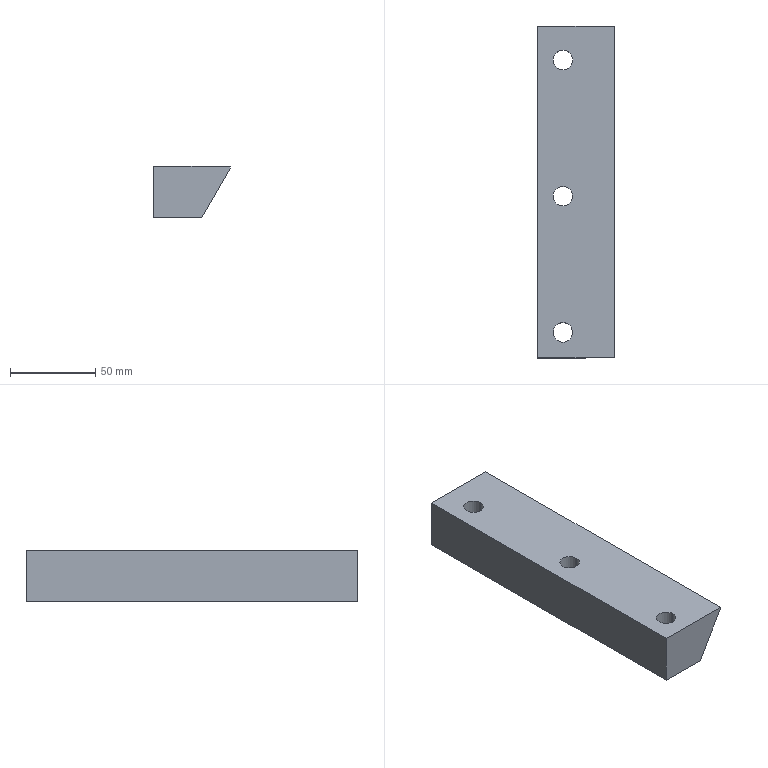Part | STEP file | NGAM TRUOT | 1 solid | 13 faces | box 45 x 195 x 30 mm | volume 206561 mm3 | plane 7 | cylinder 6 | commonest cylinder face diameters 11.5 x6
STEP:
#1=CARTESIAN_POINT('',(0.,0.,0.));
#2=DIRECTION('',(0.,0.,1.));
#3=DIRECTION('',(1.,0.,0.));
#4=AXIS2_PLACEMENT_3D('',#1,#2,#3);
#5=CARTESIAN_POINT('',(20.55,180.,0.));
#6=VERTEX_POINT('',#5);
#7=CARTESIAN_POINT('',(20.55,180.,30.));
#8=VERTEX_POINT('',#7);
#9=CARTESIAN_POINT('',(20.55,180.,0.));
#10=DIRECTION('',(0.,0.,1.));
#11=VECTOR('',#10,1.);
#12=LINE('',#9,#11);
#13=CARTESIAN_POINT('',(14.8,180.,0.));
#14=DIRECTION('',(0.,0.,1.));
#15=DIRECTION('',(1.,0.,0.));
#16=AXIS2_PLACEMENT_3D('',#13,#14,#15);
#17=CYLINDRICAL_SURFACE('',#16,5.75);
#18=CARTESIAN_POINT('',(6.283,0.));
#19=DIRECTION('',(0.,1.));
#20=VECTOR('',#19,1.);
#21=LINE('',#18,#20);
#22=(GEOMETRIC_REPRESENTATION_CONTEXT(2)PARAMETRIC_REPRESENTATION_CONTEXT()REPRESENTATION_CONTEXT('',''));
#23=DEFINITIONAL_REPRESENTATION('',(#21),#22);
#24=PCURVE('',#17,#23);
#25=CARTESIAN_POINT('',(14.8,180.,0.));
#26=DIRECTION('',(0.,0.,1.));
#27=DIRECTION('',(1.,0.,0.));
#28=AXIS2_PLACEMENT_3D('',#25,#26,#27);
#29=CYLINDRICAL_SURFACE('',#28,5.75);
#30=CARTESIAN_POINT('',(0.,0.));
#31=DIRECTION('',(0.,1.));
#32=VECTOR('',#31,1.);
#33=LINE('',#30,#32);
#34=(GEOMETRIC_REPRESENTATION_CONTEXT(2)PARAMETRIC_REPRESENTATION_CONTEXT()REPRESENTATION_CONTEXT('',''));
#35=DEFINITIONAL_REPRESENTATION('',(#33),#34);
#36=PCURVE('',#29,#35);
#37=SURFACE_CURVE('',#12,(#24,#36),.PCURVE_S1.);
#38=EDGE_CURVE('',#6,#8,#37,.T.);
#39=ORIENTED_EDGE('',*,*,#38,.T.);
#40=CARTESIAN_POINT('',(9.05,180.,30.));
#41=VERTEX_POINT('',#40);
#42=CARTESIAN_POINT('',(14.8,180.,30.));
#43=DIRECTION('',(0.,0.,-1.));
#44=DIRECTION('',(1.,0.,0.));
#45=AXIS2_PLACEMENT_3D('',#42,#43,#44);
#46=CIRCLE('',#45,5.75);
#47=CARTESIAN_POINT('',(6.283,30.));
#48=DIRECTION('',(-1.,0.));
#49=VECTOR('',#48,1.);
#50=LINE('',#47,#49);
#51=(GEOMETRIC_REPRESENTATION_CONTEXT(2)PARAMETRIC_REPRESENTATION_CONTEXT()REPRESENTATION_CONTEXT('',''));
#52=DEFINITIONAL_REPRESENTATION('',(#50),#51);
#53=PCURVE('',#17,#52);
#54=CARTESIAN_POINT('',(22.5,100.,30.));
#55=DIRECTION('',(0.,0.,1.));
#56=DIRECTION('',(1.,0.,0.));
#57=AXIS2_PLACEMENT_3D('',#54,#55,#56);
#58=PLANE('',#57);
#59=CARTESIAN_POINT('',(-1.95,80.));
#60=CARTESIAN_POINT('',(-1.95,70.041));
#61=CARTESIAN_POINT('',(-10.575,75.02));
#62=CARTESIAN_POINT('',(-19.2,80.));
#63=CARTESIAN_POINT('',(-10.575,84.98));
#64=CARTESIAN_POINT('',(-1.95,89.959));
#65=CARTESIAN_POINT('',(-1.95,80.));
#66=(BOUNDED_CURVE()B_SPLINE_CURVE(2,(#59,#60,#61,#62,#63,#64,#65),.UNSPECIFIED.,.T.,.F.)B_SPLINE_CURVE_WITH_KNOTS((1,2,2,2,2,1),(-2.094,0.,2.094,4.189,6.283,8.378),.UNSPECIFIED.)CURVE()GEOMETRIC_REPRESENTATION_ITEM()RATIONAL_B_SPLINE_CURVE((1.,0.5,1.,0.5,1.,0.5,1.))REPRESENTATION_ITEM(''));
#67=(GEOMETRIC_REPRESENTATION_CONTEXT(2)PARAMETRIC_REPRESENTATION_CONTEXT()REPRESENTATION_CONTEXT('',''));
#68=DEFINITIONAL_REPRESENTATION('',(#66),#67);
#69=PCURVE('',#58,#68);
#70=SURFACE_CURVE('',#46,(#53,#69),.PCURVE_S1.);
#71=EDGE_CURVE('',#8,#41,#70,.T.);
#72=ORIENTED_EDGE('',*,*,#71,.T.);
#73=CARTESIAN_POINT('',(9.05,180.,0.));
#74=VERTEX_POINT('',#73);
#75=CARTESIAN_POINT('',(9.05,180.,0.));
#76=DIRECTION('',(0.,0.,1.));
#77=VECTOR('',#76,1.);
#78=LINE('',#75,#77);
#79=CARTESIAN_POINT('',(3.142,0.));
#80=DIRECTION('',(0.,1.));
#81=VECTOR('',#80,1.);
#82=LINE('',#79,#81);
#83=(GEOMETRIC_REPRESENTATION_CONTEXT(2)PARAMETRIC_REPRESENTATION_CONTEXT()REPRESENTATION_CONTEXT('',''));
#84=DEFINITIONAL_REPRESENTATION('',(#82),#83);
#85=PCURVE('',#17,#84);
#86=CARTESIAN_POINT('',(3.142,0.));
#87=DIRECTION('',(0.,1.));
#88=VECTOR('',#87,1.);
#89=LINE('',#86,#88);
#90=(GEOMETRIC_REPRESENTATION_CONTEXT(2)PARAMETRIC_REPRESENTATION_CONTEXT()REPRESENTATION_CONTEXT('',''));
#91=DEFINITIONAL_REPRESENTATION('',(#89),#90);
#92=PCURVE('',#29,#91);
#93=SURFACE_CURVE('',#78,(#85,#92),.PCURVE_S1.);
#94=EDGE_CURVE('',#74,#41,#93,.T.);
#95=ORIENTED_EDGE('',*,*,#94,.F.);
#96=CARTESIAN_POINT('',(14.8,180.,0.));
#97=DIRECTION('',(0.,0.,1.));
#98=DIRECTION('',(1.,0.,0.));
#99=AXIS2_PLACEMENT_3D('',#96,#97,#98);
#100=CIRCLE('',#99,5.75);
#101=CARTESIAN_POINT('',(0.,0.));
#102=DIRECTION('',(1.,0.));
#103=VECTOR('',#102,1.);
#104=LINE('',#101,#103);
#105=(GEOMETRIC_REPRESENTATION_CONTEXT(2)PARAMETRIC_REPRESENTATION_CONTEXT()REPRESENTATION_CONTEXT('',''));
#106=DEFINITIONAL_REPRESENTATION('',(#104),#105);
#107=PCURVE('',#17,#106);
#108=CARTESIAN_POINT('',(22.5,100.,0.));
#109=DIRECTION('',(0.,0.,1.));
#110=DIRECTION('',(1.,0.,0.));
#111=AXIS2_PLACEMENT_3D('',#108,#109,#110);
#112=PLANE('',#111);
#113=CARTESIAN_POINT('',(-7.7,80.));
#114=DIRECTION('',(1.,0.));
#115=AXIS2_PLACEMENT_2D('',#113,#114);
#116=CIRCLE('',#115,5.75);
#117=(GEOMETRIC_REPRESENTATION_CONTEXT(2)PARAMETRIC_REPRESENTATION_CONTEXT()REPRESENTATION_CONTEXT('',''));
#118=DEFINITIONAL_REPRESENTATION('',(#116),#117);
#119=PCURVE('',#112,#118);
#120=SURFACE_CURVE('',#100,(#107,#119),.PCURVE_S1.);
#121=EDGE_CURVE('',#74,#6,#120,.T.);
#122=ORIENTED_EDGE('',*,*,#121,.T.);
#123=EDGE_LOOP('',(#39,#72,#95,#122));
#124=FACE_BOUND('',#123,.F.);
#125=ADVANCED_FACE('',(#124),#17,.F.);
#126=CARTESIAN_POINT('',(20.55,100.,0.));
#127=VERTEX_POINT('',#126);
#128=CARTESIAN_POINT('',(20.55,100.,30.));
#129=VERTEX_POINT('',#128);
#130=CARTESIAN_POINT('',(20.55,100.,0.));
#131=DIRECTION('',(0.,0.,1.));
#132=VECTOR('',#131,1.);
#133=LINE('',#130,#132);
#134=CARTESIAN_POINT('',(14.8,100.,0.));
#135=DIRECTION('',(0.,0.,1.));
#136=DIRECTION('',(1.,0.,0.));
#137=AXIS2_PLACEMENT_3D('',#134,#135,#136);
#138=CYLINDRICAL_SURFACE('',#137,5.75);
#139=CARTESIAN_POINT('',(6.283,0.));
#140=DIRECTION('',(0.,1.));
#141=VECTOR('',#140,1.);
#142=LINE('',#139,#141);
#143=(GEOMETRIC_REPRESENTATION_CONTEXT(2)PARAMETRIC_REPRESENTATION_CONTEXT()REPRESENTATION_CONTEXT('',''));
#144=DEFINITIONAL_REPRESENTATION('',(#142),#143);
#145=PCURVE('',#138,#144);
#146=CARTESIAN_POINT('',(14.8,100.,0.));
#147=DIRECTION('',(0.,0.,1.));
#148=DIRECTION('',(1.,0.,0.));
#149=AXIS2_PLACEMENT_3D('',#146,#147,#148);
#150=CYLINDRICAL_SURFACE('',#149,5.75);
#151=CARTESIAN_POINT('',(0.,0.));
#152=DIRECTION('',(0.,1.));
#153=VECTOR('',#152,1.);
#154=LINE('',#151,#153);
#155=(GEOMETRIC_REPRESENTATION_CONTEXT(2)PARAMETRIC_REPRESENTATION_CONTEXT()REPRESENTATION_CONTEXT('',''));
#156=DEFINITIONAL_REPRESENTATION('',(#154),#155);
#157=PCURVE('',#150,#156);
#158=SURFACE_CURVE('',#133,(#145,#157),.PCURVE_S1.);
#159=EDGE_CURVE('',#127,#129,#158,.T.);
#160=ORIENTED_EDGE('',*,*,#159,.T.);
#161=CARTESIAN_POINT('',(9.05,100.,30.));
#162=VERTEX_POINT('',#161);
#163=CARTESIAN_POINT('',(14.8,100.,30.));
#164=DIRECTION('',(0.,0.,-1.));
#165=DIRECTION('',(1.,0.,0.));
#166=AXIS2_PLACEMENT_3D('',#163,#164,#165);
#167=CIRCLE('',#166,5.75);
#168=CARTESIAN_POINT('',(6.283,30.));
#169=DIRECTION('',(-1.,0.));
#170=VECTOR('',#169,1.);
#171=LINE('',#168,#170);
#172=(GEOMETRIC_REPRESENTATION_CONTEXT(2)PARAMETRIC_REPRESENTATION_CONTEXT()REPRESENTATION_CONTEXT('',''));
#173=DEFINITIONAL_REPRESENTATION('',(#171),#172);
#174=PCURVE('',#138,#173);
#175=CARTESIAN_POINT('',(-1.95,0.));
#176=CARTESIAN_POINT('',(-1.95,-9.959));
#177=CARTESIAN_POINT('',(-10.575,-4.98));
#178=CARTESIAN_POINT('',(-19.2,0.));
#179=CARTESIAN_POINT('',(-10.575,4.98));
#180=CARTESIAN_POINT('',(-1.95,9.959));
#181=CARTESIAN_POINT('',(-1.95,0.));
#182=(BOUNDED_CURVE()B_SPLINE_CURVE(2,(#175,#176,#177,#178,#179,#180,#181),.UNSPECIFIED.,.T.,.F.)B_SPLINE_CURVE_WITH_KNOTS((1,2,2,2,2,1),(-2.094,0.,2.094,4.189,6.283,8.378),.UNSPECIFIED.)CURVE()GEOMETRIC_REPRESENTATION_ITEM()RATIONAL_B_SPLINE_CURVE((1.,0.5,1.,0.5,1.,0.5,1.))REPRESENTATION_ITEM(''));
#183=(GEOMETRIC_REPRESENTATION_CONTEXT(2)PARAMETRIC_REPRESENTATION_CONTEXT()REPRESENTATION_CONTEXT('',''));
#184=DEFINITIONAL_REPRESENTATION('',(#182),#183);
#185=PCURVE('',#58,#184);
#186=SURFACE_CURVE('',#167,(#174,#185),.PCURVE_S1.);
#187=EDGE_CURVE('',#129,#162,#186,.T.);
#188=ORIENTED_EDGE('',*,*,#187,.T.);
#189=CARTESIAN_POINT('',(9.05,100.,0.));
#190=VERTEX_POINT('',#189);
#191=CARTESIAN_POINT('',(9.05,100.,0.));
#192=DIRECTION('',(0.,0.,1.));
#193=VECTOR('',#192,1.);
#194=LINE('',#191,#193);
#195=CARTESIAN_POINT('',(3.142,0.));
#196=DIRECTION('',(0.,1.));
#197=VECTOR('',#196,1.);
#198=LINE('',#195,#197);
#199=(GEOMETRIC_REPRESENTATION_CONTEXT(2)PARAMETRIC_REPRESENTATION_CONTEXT()REPRESENTATION_CONTEXT('',''));
#200=DEFINITIONAL_REPRESENTATION('',(#198),#199);
#201=PCURVE('',#138,#200);
#202=CARTESIAN_POINT('',(3.142,0.));
#203=DIRECTION('',(0.,1.));
#204=VECTOR('',#203,1.);
#205=LINE('',#202,#204);
#206=(GEOMETRIC_REPRESENTATION_CONTEXT(2)PARAMETRIC_REPRESENTATION_CONTEXT()REPRESENTATION_CONTEXT('',''));
#207=DEFINITIONAL_REPRESENTATION('',(#205),#206);
#208=PCURVE('',#150,#207);
#209=SURFACE_CURVE('',#194,(#201,#208),.PCURVE_S1.);
#210=EDGE_CURVE('',#190,#162,#209,.T.);
#211=ORIENTED_EDGE('',*,*,#210,.F.);
#212=CARTESIAN_POINT('',(14.8,100.,0.));
#213=DIRECTION('',(0.,0.,1.));
#214=DIRECTION('',(1.,0.,0.));
#215=AXIS2_PLACEMENT_3D('',#212,#213,#214);
#216=CIRCLE('',#215,5.75);
#217=CARTESIAN_POINT('',(0.,0.));
#218=DIRECTION('',(1.,0.));
#219=VECTOR('',#218,1.);
#220=LINE('',#217,#219);
#221=(GEOMETRIC_REPRESENTATION_CONTEXT(2)PARAMETRIC_REPRESENTATION_CONTEXT()REPRESENTATION_CONTEXT('',''));
#222=DEFINITIONAL_REPRESENTATION('',(#220),#221);
#223=PCURVE('',#138,#222);
#224=CARTESIAN_POINT('',(-7.7,0.));
#225=DIRECTION('',(1.,0.));
#226=AXIS2_PLACEMENT_2D('',#224,#225);
#227=CIRCLE('',#226,5.75);
#228=(GEOMETRIC_REPRESENTATION_CONTEXT(2)PARAMETRIC_REPRESENTATION_CONTEXT()REPRESENTATION_CONTEXT('',''));
#229=DEFINITIONAL_REPRESENTATION('',(#227),#228);
#230=PCURVE('',#112,#229);
#231=SURFACE_CURVE('',#216,(#223,#230),.PCURVE_S1.);
#232=EDGE_CURVE('',#190,#127,#231,.T.);
#233=ORIENTED_EDGE('',*,*,#232,.T.);
#234=EDGE_LOOP('',(#160,#188,#211,#233));
#235=FACE_BOUND('',#234,.F.);
#236=ADVANCED_FACE('',(#235),#138,.F.);
#237=CARTESIAN_POINT('',(20.55,20.,0.));
#238=VERTEX_POINT('',#237);
#239=CARTESIAN_POINT('',(20.55,20.,30.));
#240=VERTEX_POINT('',#239);
#241=CARTESIAN_POINT('',(20.55,20.,0.));
#242=DIRECTION('',(0.,0.,1.));
#243=VECTOR('',#242,1.);
#244=LINE('',#241,#243);
#245=CARTESIAN_POINT('',(14.8,20.,0.));
#246=DIRECTION('',(0.,0.,1.));
#247=DIRECTION('',(1.,0.,0.));
#248=AXIS2_PLACEMENT_3D('',#245,#246,#247);
#249=CYLINDRICAL_SURFACE('',#248,5.75);
#250=CARTESIAN_POINT('',(6.283,0.));
#251=DIRECTION('',(0.,1.));
#252=VECTOR('',#251,1.);
#253=LINE('',#250,#252);
#254=(GEOMETRIC_REPRESENTATION_CONTEXT(2)PARAMETRIC_REPRESENTATION_CONTEXT()REPRESENTATION_CONTEXT('',''));
#255=DEFINITIONAL_REPRESENTATION('',(#253),#254);
#256=PCURVE('',#249,#255);
#257=CARTESIAN_POINT('',(14.8,20.,0.));
#258=DIRECTION('',(0.,0.,1.));
#259=DIRECTION('',(1.,0.,0.));
#260=AXIS2_PLACEMENT_3D('',#257,#258,#259);
#261=CYLINDRICAL_SURFACE('',#260,5.75);
#262=CARTESIAN_POINT('',(0.,0.));
#263=DIRECTION('',(0.,1.));
#264=VECTOR('',#263,1.);
#265=LINE('',#262,#264);
#266=(GEOMETRIC_REPRESENTATION_CONTEXT(2)PARAMETRIC_REPRESENTATION_CONTEXT()REPRESENTATION_CONTEXT('',''));
#267=DEFINITIONAL_REPRESENTATION('',(#265),#266);
#268=PCURVE('',#261,#267);
#269=SURFACE_CURVE('',#244,(#256,#268),.PCURVE_S1.);
#270=EDGE_CURVE('',#238,#240,#269,.T.);
#271=ORIENTED_EDGE('',*,*,#270,.T.);
#272=CARTESIAN_POINT('',(9.05,20.,30.));
#273=VERTEX_POINT('',#272);
#274=CARTESIAN_POINT('',(14.8,20.,30.));
#275=DIRECTION('',(0.,0.,-1.));
#276=DIRECTION('',(1.,0.,0.));
#277=AXIS2_PLACEMENT_3D('',#274,#275,#276);
#278=CIRCLE('',#277,5.75);
#279=CARTESIAN_POINT('',(6.283,30.));
#280=DIRECTION('',(-1.,0.));
#281=VECTOR('',#280,1.);
#282=LINE('',#279,#281);
#283=(GEOMETRIC_REPRESENTATION_CONTEXT(2)PARAMETRIC_REPRESENTATION_CONTEXT()REPRESENTATION_CONTEXT('',''));
#284=DEFINITIONAL_REPRESENTATION('',(#282),#283);
#285=PCURVE('',#249,#284);
#286=CARTESIAN_POINT('',(-1.95,-80.));
#287=CARTESIAN_POINT('',(-1.95,-89.959));
#288=CARTESIAN_POINT('',(-10.575,-84.98));
#289=CARTESIAN_POINT('',(-19.2,-80.));
#290=CARTESIAN_POINT('',(-10.575,-75.02));
#291=CARTESIAN_POINT('',(-1.95,-70.041));
#292=CARTESIAN_POINT('',(-1.95,-80.));
#293=(BOUNDED_CURVE()B_SPLINE_CURVE(2,(#286,#287,#288,#289,#290,#291,#292),.UNSPECIFIED.,.T.,.F.)B_SPLINE_CURVE_WITH_KNOTS((1,2,2,2,2,1),(-2.094,0.,2.094,4.189,6.283,8.378),.UNSPECIFIED.)CURVE()GEOMETRIC_REPRESENTATION_ITEM()RATIONAL_B_SPLINE_CURVE((1.,0.5,1.,0.5,1.,0.5,1.))REPRESENTATION_ITEM(''));
#294=(GEOMETRIC_REPRESENTATION_CONTEXT(2)PARAMETRIC_REPRESENTATION_CONTEXT()REPRESENTATION_CONTEXT('',''));
#295=DEFINITIONAL_REPRESENTATION('',(#293),#294);
#296=PCURVE('',#58,#295);
#297=SURFACE_CURVE('',#278,(#285,#296),.PCURVE_S1.);
#298=EDGE_CURVE('',#240,#273,#297,.T.);
#299=ORIENTED_EDGE('',*,*,#298,.T.);
#300=CARTESIAN_POINT('',(9.05,20.,0.));
#301=VERTEX_POINT('',#300);
#302=CARTESIAN_POINT('',(9.05,20.,0.));
#303=DIRECTION('',(0.,0.,1.));
#304=VECTOR('',#303,1.);
#305=LINE('',#302,#304);
#306=CARTESIAN_POINT('',(3.142,0.));
#307=DIRECTION('',(0.,1.));
#308=VECTOR('',#307,1.);
#309=LINE('',#306,#308);
#310=(GEOMETRIC_REPRESENTATION_CONTEXT(2)PARAMETRIC_REPRESENTATION_CONTEXT()REPRESENTATION_CONTEXT('',''));
#311=DEFINITIONAL_REPRESENTATION('',(#309),#310);
#312=PCURVE('',#249,#311);
#313=CARTESIAN_POINT('',(3.142,0.));
#314=DIRECTION('',(0.,1.));
#315=VECTOR('',#314,1.);
#316=LINE('',#313,#315);
#317=(GEOMETRIC_REPRESENTATION_CONTEXT(2)PARAMETRIC_REPRESENTATION_CONTEXT()REPRESENTATION_CONTEXT('',''));
#318=DEFINITIONAL_REPRESENTATION('',(#316),#317);
#319=PCURVE('',#261,#318);
#320=SURFACE_CURVE('',#305,(#312,#319),.PCURVE_S1.);
#321=EDGE_CURVE('',#301,#273,#320,.T.);
#322=ORIENTED_EDGE('',*,*,#321,.F.);
#323=CARTESIAN_POINT('',(14.8,20.,0.));
#324=DIRECTION('',(0.,0.,1.));
#325=DIRECTION('',(1.,0.,0.));
#326=AXIS2_PLACEMENT_3D('',#323,#324,#325);
#327=CIRCLE('',#326,5.75);
#328=CARTESIAN_POINT('',(0.,0.));
#329=DIRECTION('',(1.,0.));
#330=VECTOR('',#329,1.);
#331=LINE('',#328,#330);
#332=(GEOMETRIC_REPRESENTATION_CONTEXT(2)PARAMETRIC_REPRESENTATION_CONTEXT()REPRESENTATION_CONTEXT('',''));
#333=DEFINITIONAL_REPRESENTATION('',(#331),#332);
#334=PCURVE('',#249,#333);
#335=CARTESIAN_POINT('',(-7.7,-80.));
#336=DIRECTION('',(1.,0.));
#337=AXIS2_PLACEMENT_2D('',#335,#336);
#338=CIRCLE('',#337,5.75);
#339=(GEOMETRIC_REPRESENTATION_CONTEXT(2)PARAMETRIC_REPRESENTATION_CONTEXT()REPRESENTATION_CONTEXT('',''));
#340=DEFINITIONAL_REPRESENTATION('',(#338),#339);
#341=PCURVE('',#112,#340);
#342=SURFACE_CURVE('',#327,(#334,#341),.PCURVE_S1.);
#343=EDGE_CURVE('',#301,#238,#342,.T.);
#344=ORIENTED_EDGE('',*,*,#343,.T.);
#345=EDGE_LOOP('',(#271,#299,#322,#344));
#346=FACE_BOUND('',#345,.F.);
#347=ADVANCED_FACE('',(#346),#249,.F.);
#348=ORIENTED_EDGE('',*,*,#71,.T.);
#349=CARTESIAN_POINT('',(14.8,180.,30.));
#350=DIRECTION('',(0.,0.,-1.));
#351=DIRECTION('',(1.,0.,0.));
#352=AXIS2_PLACEMENT_3D('',#349,#350,#351);
#353=CIRCLE('',#352,5.75);
#354=CARTESIAN_POINT('',(-1.95,80.));
#355=CARTESIAN_POINT('',(-1.95,70.041));
#356=CARTESIAN_POINT('',(-10.575,75.02));
#357=CARTESIAN_POINT('',(-19.2,80.));
#358=CARTESIAN_POINT('',(-10.575,84.98));
#359=CARTESIAN_POINT('',(-1.95,89.959));
#360=CARTESIAN_POINT('',(-1.95,80.));
#361=(BOUNDED_CURVE()B_SPLINE_CURVE(2,(#354,#355,#356,#357,#358,#359,#360),.UNSPECIFIED.,.T.,.F.)B_SPLINE_CURVE_WITH_KNOTS((1,2,2,2,2,1),(-2.094,0.,2.094,4.189,6.283,8.378),.UNSPECIFIED.)CURVE()GEOMETRIC_REPRESENTATION_ITEM()RATIONAL_B_SPLINE_CURVE((1.,0.5,1.,0.5,1.,0.5,1.))REPRESENTATION_ITEM(''));
#362=(GEOMETRIC_REPRESENTATION_CONTEXT(2)PARAMETRIC_REPRESENTATION_CONTEXT()REPRESENTATION_CONTEXT('',''));
#363=DEFINITIONAL_REPRESENTATION('',(#361),#362);
#364=PCURVE('',#58,#363);
#365=CARTESIAN_POINT('',(6.283,30.));
#366=DIRECTION('',(-1.,0.));
#367=VECTOR('',#366,1.);
#368=LINE('',#365,#367);
#369=(GEOMETRIC_REPRESENTATION_CONTEXT(2)PARAMETRIC_REPRESENTATION_CONTEXT()REPRESENTATION_CONTEXT('',''));
#370=DEFINITIONAL_REPRESENTATION('',(#368),#369);
#371=PCURVE('',#29,#370);
#372=SURFACE_CURVE('',#353,(#364,#371),.PCURVE_S1.);
#373=EDGE_CURVE('',#41,#8,#372,.T.);
#374=ORIENTED_EDGE('',*,*,#373,.T.);
#375=EDGE_LOOP('',(#348,#374));
#376=FACE_BOUND('',#375,.T.);
#377=ORIENTED_EDGE('',*,*,#187,.T.);
#378=CARTESIAN_POINT('',(14.8,100.,30.));
#379=DIRECTION('',(0.,0.,-1.));
#380=DIRECTION('',(1.,0.,0.));
#381=AXIS2_PLACEMENT_3D('',#378,#379,#380);
#382=CIRCLE('',#381,5.75);
#383=CARTESIAN_POINT('',(-1.95,0.));
#384=CARTESIAN_POINT('',(-1.95,-9.959));
#385=CARTESIAN_POINT('',(-10.575,-4.98));
#386=CARTESIAN_POINT('',(-19.2,0.));
#387=CARTESIAN_POINT('',(-10.575,4.98));
#388=CARTESIAN_POINT('',(-1.95,9.959));
#389=CARTESIAN_POINT('',(-1.95,0.));
#390=(BOUNDED_CURVE()B_SPLINE_CURVE(2,(#383,#384,#385,#386,#387,#388,#389),.UNSPECIFIED.,.T.,.F.)B_SPLINE_CURVE_WITH_KNOTS((1,2,2,2,2,1),(-2.094,0.,2.094,4.189,6.283,8.378),.UNSPECIFIED.)CURVE()GEOMETRIC_REPRESENTATION_ITEM()RATIONAL_B_SPLINE_CURVE((1.,0.5,1.,0.5,1.,0.5,1.))REPRESENTATION_ITEM(''));
#391=(GEOMETRIC_REPRESENTATION_CONTEXT(2)PARAMETRIC_REPRESENTATION_CONTEXT()REPRESENTATION_CONTEXT('',''));
#392=DEFINITIONAL_REPRESENTATION('',(#390),#391);
#393=PCURVE('',#58,#392);
#394=CARTESIAN_POINT('',(6.283,30.));
#395=DIRECTION('',(-1.,0.));
#396=VECTOR('',#395,1.);
#397=LINE('',#394,#396);
#398=(GEOMETRIC_REPRESENTATION_CONTEXT(2)PARAMETRIC_REPRESENTATION_CONTEXT()REPRESENTATION_CONTEXT('',''));
#399=DEFINITIONAL_REPRESENTATION('',(#397),#398);
#400=PCURVE('',#150,#399);
#401=SURFACE_CURVE('',#382,(#393,#400),.PCURVE_S1.);
#402=EDGE_CURVE('',#162,#129,#401,.T.);
#403=ORIENTED_EDGE('',*,*,#402,.T.);
#404=EDGE_LOOP('',(#377,#403));
#405=FACE_BOUND('',#404,.T.);
#406=ORIENTED_EDGE('',*,*,#298,.T.);
#407=CARTESIAN_POINT('',(14.8,20.,30.));
#408=DIRECTION('',(0.,0.,-1.));
#409=DIRECTION('',(1.,0.,0.));
#410=AXIS2_PLACEMENT_3D('',#407,#408,#409);
#411=CIRCLE('',#410,5.75);
#412=CARTESIAN_POINT('',(-1.95,-80.));
#413=CARTESIAN_POINT('',(-1.95,-89.959));
#414=CARTESIAN_POINT('',(-10.575,-84.98));
#415=CARTESIAN_POINT('',(-19.2,-80.));
#416=CARTESIAN_POINT('',(-10.575,-75.02));
#417=CARTESIAN_POINT('',(-1.95,-70.041));
#418=CARTESIAN_POINT('',(-1.95,-80.));
#419=(BOUNDED_CURVE()B_SPLINE_CURVE(2,(#412,#413,#414,#415,#416,#417,#418),.UNSPECIFIED.,.T.,.F.)B_SPLINE_CURVE_WITH_KNOTS((1,2,2,2,2,1),(-2.094,0.,2.094,4.189,6.283,8.378),.UNSPECIFIED.)CURVE()GEOMETRIC_REPRESENTATION_ITEM()RATIONAL_B_SPLINE_CURVE((1.,0.5,1.,0.5,1.,0.5,1.))REPRESENTATION_ITEM(''));
#420=(GEOMETRIC_REPRESENTATION_CONTEXT(2)PARAMETRIC_REPRESENTATION_CONTEXT()REPRESENTATION_CONTEXT('',''));
#421=DEFINITIONAL_REPRESENTATION('',(#419),#420);
#422=PCURVE('',#58,#421);
#423=CARTESIAN_POINT('',(6.283,30.));
#424=DIRECTION('',(-1.,0.));
#425=VECTOR('',#424,1.);
#426=LINE('',#423,#425);
#427=(GEOMETRIC_REPRESENTATION_CONTEXT(2)PARAMETRIC_REPRESENTATION_CONTEXT()REPRESENTATION_CONTEXT('',''));
#428=DEFINITIONAL_REPRESENTATION('',(#426),#427);
#429=PCURVE('',#261,#428);
#430=SURFACE_CURVE('',#411,(#422,#429),.PCURVE_S1.);
#431=EDGE_CURVE('',#273,#240,#430,.T.);
#432=ORIENTED_EDGE('',*,*,#431,.T.);
#433=EDGE_LOOP('',(#406,#432));
#434=FACE_BOUND('',#433,.T.);
#435=CARTESIAN_POINT('',(45.,200.,30.));
#436=VERTEX_POINT('',#435);
#437=CARTESIAN_POINT('',(0.,200.,30.));
#438=VERTEX_POINT('',#437);
#439=CARTESIAN_POINT('',(22.5,200.,30.));
#440=DIRECTION('',(-1.,0.,0.));
#441=VECTOR('',#440,1.);
#442=LINE('',#439,#441);
#443=CARTESIAN_POINT('',(0.,100.));
#444=DIRECTION('',(-1.,0.));
#445=VECTOR('',#444,1.);
#446=LINE('',#443,#445);
#447=(GEOMETRIC_REPRESENTATION_CONTEXT(2)PARAMETRIC_REPRESENTATION_CONTEXT()REPRESENTATION_CONTEXT('',''));
#448=DEFINITIONAL_REPRESENTATION('',(#446),#447);
#449=PCURVE('',#58,#448);
#450=CARTESIAN_POINT('',(0.,200.,0.));
#451=DIRECTION('',(0.,1.,0.));
#452=DIRECTION('',(0.,0.,1.));
#453=AXIS2_PLACEMENT_3D('',#450,#451,#452);
#454=PLANE('',#453);
#455=CARTESIAN_POINT('',(30.,22.5));
#456=DIRECTION('',(0.,-1.));
#457=VECTOR('',#456,1.);
#458=LINE('',#455,#457);
#459=(GEOMETRIC_REPRESENTATION_CONTEXT(2)PARAMETRIC_REPRESENTATION_CONTEXT()REPRESENTATION_CONTEXT('',''));
#460=DEFINITIONAL_REPRESENTATION('',(#458),#459);
#461=PCURVE('',#454,#460);
#462=SURFACE_CURVE('',#442,(#449,#461),.PCURVE_S1.);
#463=EDGE_CURVE('',#436,#438,#462,.T.);
#464=ORIENTED_EDGE('',*,*,#463,.T.);
#465=CARTESIAN_POINT('',(0.,5.,30.));
#466=VERTEX_POINT('',#465);
#467=CARTESIAN_POINT('',(0.,100.,30.));
#468=DIRECTION('',(0.,-1.,0.));
#469=VECTOR('',#468,1.);
#470=LINE('',#467,#469);
#471=CARTESIAN_POINT('',(-22.5,0.));
#472=DIRECTION('',(0.,-1.));
#473=VECTOR('',#472,1.);
#474=LINE('',#471,#473);
#475=(GEOMETRIC_REPRESENTATION_CONTEXT(2)PARAMETRIC_REPRESENTATION_CONTEXT()REPRESENTATION_CONTEXT('',''));
#476=DEFINITIONAL_REPRESENTATION('',(#474),#475);
#477=PCURVE('',#58,#476);
#478=CARTESIAN_POINT('',(0.,0.,0.));
#479=DIRECTION('',(-1.,0.,0.));
#480=DIRECTION('',(0.,0.,1.));
#481=AXIS2_PLACEMENT_3D('',#478,#479,#480);
#482=PLANE('',#481);
#483=CARTESIAN_POINT('',(30.,100.));
#484=DIRECTION('',(0.,-1.));
#485=VECTOR('',#484,1.);
#486=LINE('',#483,#485);
#487=(GEOMETRIC_REPRESENTATION_CONTEXT(2)PARAMETRIC_REPRESENTATION_CONTEXT()REPRESENTATION_CONTEXT('',''));
#488=DEFINITIONAL_REPRESENTATION('',(#486),#487);
#489=PCURVE('',#482,#488);
#490=SURFACE_CURVE('',#470,(#477,#489),.PCURVE_S1.);
#491=EDGE_CURVE('',#438,#466,#490,.T.);
#492=ORIENTED_EDGE('',*,*,#491,.T.);
#493=CARTESIAN_POINT('',(45.,5.,30.));
#494=VERTEX_POINT('',#493);
#495=CARTESIAN_POINT('',(22.5,5.,30.));
#496=DIRECTION('',(1.,0.,0.));
#497=VECTOR('',#496,1.);
#498=LINE('',#495,#497);
#499=CARTESIAN_POINT('',(0.,-95.));
#500=DIRECTION('',(1.,0.));
#501=VECTOR('',#500,1.);
#502=LINE('',#499,#501);
#503=(GEOMETRIC_REPRESENTATION_CONTEXT(2)PARAMETRIC_REPRESENTATION_CONTEXT()REPRESENTATION_CONTEXT('',''));
#504=DEFINITIONAL_REPRESENTATION('',(#502),#503);
#505=PCURVE('',#58,#504);
#506=CARTESIAN_POINT('',(19.48,5.,16.807));
#507=DIRECTION('',(0.,1.,0.));
#508=DIRECTION('',(0.,0.,1.));
#509=AXIS2_PLACEMENT_3D('',#506,#507,#508);
#510=PLANE('',#509);
#511=CARTESIAN_POINT('',(13.193,3.02));
#512=DIRECTION('',(0.,1.));
#513=VECTOR('',#512,1.);
#514=LINE('',#511,#513);
#515=(GEOMETRIC_REPRESENTATION_CONTEXT(2)PARAMETRIC_REPRESENTATION_CONTEXT()REPRESENTATION_CONTEXT('',''));
#516=DEFINITIONAL_REPRESENTATION('',(#514),#515);
#517=PCURVE('',#510,#516);
#518=SURFACE_CURVE('',#498,(#505,#517),.PCURVE_S1.);
#519=EDGE_CURVE('',#466,#494,#518,.T.);
#520=ORIENTED_EDGE('',*,*,#519,.T.);
#521=CARTESIAN_POINT('',(45.,100.,30.));
#522=DIRECTION('',(0.,1.,0.));
#523=VECTOR('',#522,1.);
#524=LINE('',#521,#523);
#525=CARTESIAN_POINT('',(22.5,0.));
#526=DIRECTION('',(0.,1.));
#527=VECTOR('',#526,1.);
#528=LINE('',#525,#527);
#529=(GEOMETRIC_REPRESENTATION_CONTEXT(2)PARAMETRIC_REPRESENTATION_CONTEXT()REPRESENTATION_CONTEXT('',''));
#530=DEFINITIONAL_REPRESENTATION('',(#528),#529);
#531=PCURVE('',#58,#530);
#532=CARTESIAN_POINT('',(45.,200.,0.));
#533=DIRECTION('',(1.,0.,0.));
#534=DIRECTION('',(0.,0.,-1.));
#535=AXIS2_PLACEMENT_3D('',#532,#533,#534);
#536=PLANE('',#535);
#537=CARTESIAN_POINT('',(-30.,-100.));
#538=DIRECTION('',(0.,1.));
#539=VECTOR('',#538,1.);
#540=LINE('',#537,#539);
#541=(GEOMETRIC_REPRESENTATION_CONTEXT(2)PARAMETRIC_REPRESENTATION_CONTEXT()REPRESENTATION_CONTEXT('',''));
#542=DEFINITIONAL_REPRESENTATION('',(#540),#541);
#543=PCURVE('',#536,#542);
#544=SURFACE_CURVE('',#524,(#531,#543),.PCURVE_S1.);
#545=EDGE_CURVE('',#494,#436,#544,.T.);
#546=ORIENTED_EDGE('',*,*,#545,.T.);
#547=EDGE_LOOP('',(#464,#492,#520,#546));
#548=FACE_BOUND('',#547,.T.);
#549=ADVANCED_FACE('',(#376,#405,#434,#548),#58,.T.);
#550=ORIENTED_EDGE('',*,*,#373,.T.);
#551=ORIENTED_EDGE('',*,*,#38,.F.);
#552=CARTESIAN_POINT('',(14.8,180.,0.));
#553=DIRECTION('',(0.,0.,1.));
#554=DIRECTION('',(1.,0.,0.));
#555=AXIS2_PLACEMENT_3D('',#552,#553,#554);
#556=CIRCLE('',#555,5.75);
#557=CARTESIAN_POINT('',(0.,0.));
#558=DIRECTION('',(1.,0.));
#559=VECTOR('',#558,1.);
#560=LINE('',#557,#559);
#561=(GEOMETRIC_REPRESENTATION_CONTEXT(2)PARAMETRIC_REPRESENTATION_CONTEXT()REPRESENTATION_CONTEXT('',''));
#562=DEFINITIONAL_REPRESENTATION('',(#560),#561);
#563=PCURVE('',#29,#562);
#564=CARTESIAN_POINT('',(-7.7,80.));
#565=DIRECTION('',(1.,0.));
#566=AXIS2_PLACEMENT_2D('',#564,#565);
#567=CIRCLE('',#566,5.75);
#568=(GEOMETRIC_REPRESENTATION_CONTEXT(2)PARAMETRIC_REPRESENTATION_CONTEXT()REPRESENTATION_CONTEXT('',''));
#569=DEFINITIONAL_REPRESENTATION('',(#567),#568);
#570=PCURVE('',#112,#569);
#571=SURFACE_CURVE('',#556,(#563,#570),.PCURVE_S1.);
#572=EDGE_CURVE('',#6,#74,#571,.T.);
#573=ORIENTED_EDGE('',*,*,#572,.T.);
#574=ORIENTED_EDGE('',*,*,#94,.T.);
#575=EDGE_LOOP('',(#550,#551,#573,#574));
#576=FACE_BOUND('',#575,.F.);
#577=ADVANCED_FACE('',(#576),#29,.F.);
#578=ORIENTED_EDGE('',*,*,#402,.T.);
#579=ORIENTED_EDGE('',*,*,#159,.F.);
#580=CARTESIAN_POINT('',(14.8,100.,0.));
#581=DIRECTION('',(0.,0.,1.));
#582=DIRECTION('',(1.,0.,0.));
#583=AXIS2_PLACEMENT_3D('',#580,#581,#582);
#584=CIRCLE('',#583,5.75);
#585=CARTESIAN_POINT('',(0.,0.));
#586=DIRECTION('',(1.,0.));
#587=VECTOR('',#586,1.);
#588=LINE('',#585,#587);
#589=(GEOMETRIC_REPRESENTATION_CONTEXT(2)PARAMETRIC_REPRESENTATION_CONTEXT()REPRESENTATION_CONTEXT('',''));
#590=DEFINITIONAL_REPRESENTATION('',(#588),#589);
#591=PCURVE('',#150,#590);
#592=CARTESIAN_POINT('',(-7.7,0.));
#593=DIRECTION('',(1.,0.));
#594=AXIS2_PLACEMENT_2D('',#592,#593);
#595=CIRCLE('',#594,5.75);
#596=(GEOMETRIC_REPRESENTATION_CONTEXT(2)PARAMETRIC_REPRESENTATION_CONTEXT()REPRESENTATION_CONTEXT('',''));
#597=DEFINITIONAL_REPRESENTATION('',(#595),#596);
#598=PCURVE('',#112,#597);
#599=SURFACE_CURVE('',#584,(#591,#598),.PCURVE_S1.);
#600=EDGE_CURVE('',#127,#190,#599,.T.);
#601=ORIENTED_EDGE('',*,*,#600,.T.);
#602=ORIENTED_EDGE('',*,*,#210,.T.);
#603=EDGE_LOOP('',(#578,#579,#601,#602));
#604=FACE_BOUND('',#603,.F.);
#605=ADVANCED_FACE('',(#604),#150,.F.);
#606=ORIENTED_EDGE('',*,*,#431,.T.);
#607=ORIENTED_EDGE('',*,*,#270,.F.);
#608=CARTESIAN_POINT('',(14.8,20.,0.));
#609=DIRECTION('',(0.,0.,1.));
#610=DIRECTION('',(1.,0.,0.));
#611=AXIS2_PLACEMENT_3D('',#608,#609,#610);
#612=CIRCLE('',#611,5.75);
#613=CARTESIAN_POINT('',(0.,0.));
#614=DIRECTION('',(1.,0.));
#615=VECTOR('',#614,1.);
#616=LINE('',#613,#615);
#617=(GEOMETRIC_REPRESENTATION_CONTEXT(2)PARAMETRIC_REPRESENTATION_CONTEXT()REPRESENTATION_CONTEXT('',''));
#618=DEFINITIONAL_REPRESENTATION('',(#616),#617);
#619=PCURVE('',#261,#618);
#620=CARTESIAN_POINT('',(-7.7,-80.));
#621=DIRECTION('',(1.,0.));
#622=AXIS2_PLACEMENT_2D('',#620,#621);
#623=CIRCLE('',#622,5.75);
#624=(GEOMETRIC_REPRESENTATION_CONTEXT(2)PARAMETRIC_REPRESENTATION_CONTEXT()REPRESENTATION_CONTEXT('',''));
#625=DEFINITIONAL_REPRESENTATION('',(#623),#624);
#626=PCURVE('',#112,#625);
#627=SURFACE_CURVE('',#612,(#619,#626),.PCURVE_S1.);
#628=EDGE_CURVE('',#238,#301,#627,.T.);
#629=ORIENTED_EDGE('',*,*,#628,.T.);
#630=ORIENTED_EDGE('',*,*,#321,.T.);
#631=EDGE_LOOP('',(#606,#607,#629,#630));
#632=FACE_BOUND('',#631,.F.);
#633=ADVANCED_FACE('',(#632),#261,.F.);
#634=CARTESIAN_POINT('',(0.,200.,0.));
#635=VERTEX_POINT('',#634);
#636=CARTESIAN_POINT('',(0.,200.,0.));
#637=DIRECTION('',(0.,0.,-1.));
#638=VECTOR('',#637,1.);
#639=LINE('',#636,#638);
#640=CARTESIAN_POINT('',(0.,200.));
#641=DIRECTION('',(-1.,0.));
#642=VECTOR('',#641,1.);
#643=LINE('',#640,#642);
#644=(GEOMETRIC_REPRESENTATION_CONTEXT(2)PARAMETRIC_REPRESENTATION_CONTEXT()REPRESENTATION_CONTEXT('',''));
#645=DEFINITIONAL_REPRESENTATION('',(#643),#644);
#646=PCURVE('',#482,#645);
#647=CARTESIAN_POINT('',(0.,0.));
#648=DIRECTION('',(-1.,0.));
#649=VECTOR('',#648,1.);
#650=LINE('',#647,#649);
#651=(GEOMETRIC_REPRESENTATION_CONTEXT(2)PARAMETRIC_REPRESENTATION_CONTEXT()REPRESENTATION_CONTEXT('',''));
#652=DEFINITIONAL_REPRESENTATION('',(#650),#651);
#653=PCURVE('',#454,#652);
#654=SURFACE_CURVE('',#639,(#646,#653),.PCURVE_S1.);
#655=EDGE_CURVE('',#438,#635,#654,.T.);
#656=ORIENTED_EDGE('',*,*,#655,.T.);
#657=CARTESIAN_POINT('',(0.,5.,0.));
#658=VERTEX_POINT('',#657);
#659=CARTESIAN_POINT('',(0.,0.,0.));
#660=DIRECTION('',(0.,-1.,0.));
#661=VECTOR('',#660,1.);
#662=LINE('',#659,#661);
#663=CARTESIAN_POINT('',(0.,0.));
#664=DIRECTION('',(0.,-1.));
#665=VECTOR('',#664,1.);
#666=LINE('',#663,#665);
#667=(GEOMETRIC_REPRESENTATION_CONTEXT(2)PARAMETRIC_REPRESENTATION_CONTEXT()REPRESENTATION_CONTEXT('',''));
#668=DEFINITIONAL_REPRESENTATION('',(#666),#667);
#669=PCURVE('',#482,#668);
#670=CARTESIAN_POINT('',(-22.5,-100.));
#671=DIRECTION('',(0.,-1.));
#672=VECTOR('',#671,1.);
#673=LINE('',#670,#672);
#674=(GEOMETRIC_REPRESENTATION_CONTEXT(2)PARAMETRIC_REPRESENTATION_CONTEXT()REPRESENTATION_CONTEXT('',''));
#675=DEFINITIONAL_REPRESENTATION('',(#673),#674);
#676=PCURVE('',#112,#675);
#677=SURFACE_CURVE('',#662,(#669,#676),.PCURVE_S1.);
#678=EDGE_CURVE('',#635,#658,#677,.T.);
#679=ORIENTED_EDGE('',*,*,#678,.T.);
#680=CARTESIAN_POINT('',(0.,5.,0.));
#681=DIRECTION('',(0.,0.,1.));
#682=VECTOR('',#681,1.);
#683=LINE('',#680,#682);
#684=CARTESIAN_POINT('',(0.,5.));
#685=DIRECTION('',(1.,0.));
#686=VECTOR('',#685,1.);
#687=LINE('',#684,#686);
#688=(GEOMETRIC_REPRESENTATION_CONTEXT(2)PARAMETRIC_REPRESENTATION_CONTEXT()REPRESENTATION_CONTEXT('',''));
#689=DEFINITIONAL_REPRESENTATION('',(#687),#688);
#690=PCURVE('',#482,#689);
#691=CARTESIAN_POINT('',(-16.807,-19.48));
#692=DIRECTION('',(1.,0.));
#693=VECTOR('',#692,1.);
#694=LINE('',#691,#693);
#695=(GEOMETRIC_REPRESENTATION_CONTEXT(2)PARAMETRIC_REPRESENTATION_CONTEXT()REPRESENTATION_CONTEXT('',''));
#696=DEFINITIONAL_REPRESENTATION('',(#694),#695);
#697=PCURVE('',#510,#696);
#698=SURFACE_CURVE('',#683,(#690,#697),.PCURVE_S1.);
#699=EDGE_CURVE('',#658,#466,#698,.T.);
#700=ORIENTED_EDGE('',*,*,#699,.T.);
#701=ORIENTED_EDGE('',*,*,#491,.F.);
#702=EDGE_LOOP('',(#656,#679,#700,#701));
#703=FACE_BOUND('',#702,.T.);
#704=ADVANCED_FACE('',(#703),#482,.T.);
#705=ORIENTED_EDGE('',*,*,#463,.F.);
#706=CARTESIAN_POINT('',(45.,200.,29.));
#707=VERTEX_POINT('',#706);
#708=CARTESIAN_POINT('',(45.,200.,0.));
#709=DIRECTION('',(0.,0.,-1.));
#710=VECTOR('',#709,1.);
#711=LINE('',#708,#710);
#712=CARTESIAN_POINT('',(0.,45.));
#713=DIRECTION('',(-1.,0.));
#714=VECTOR('',#713,1.);
#715=LINE('',#712,#714);
#716=(GEOMETRIC_REPRESENTATION_CONTEXT(2)PARAMETRIC_REPRESENTATION_CONTEXT()REPRESENTATION_CONTEXT('',''));
#717=DEFINITIONAL_REPRESENTATION('',(#715),#716);
#718=PCURVE('',#454,#717);
#719=CARTESIAN_POINT('',(0.,0.));
#720=DIRECTION('',(1.,0.));
#721=VECTOR('',#720,1.);
#722=LINE('',#719,#721);
#723=(GEOMETRIC_REPRESENTATION_CONTEXT(2)PARAMETRIC_REPRESENTATION_CONTEXT()REPRESENTATION_CONTEXT('',''));
#724=DEFINITIONAL_REPRESENTATION('',(#722),#723);
#725=PCURVE('',#536,#724);
#726=SURFACE_CURVE('',#711,(#718,#725),.PCURVE_S1.);
#727=EDGE_CURVE('',#436,#707,#726,.T.);
#728=ORIENTED_EDGE('',*,*,#727,.T.);
#729=CARTESIAN_POINT('',(28.257,200.,0.));
#730=VERTEX_POINT('',#729);
#731=CARTESIAN_POINT('',(45.,200.,29.));
#732=DIRECTION('',(-0.5,0.,-0.866));
#733=VECTOR('',#732,1.);
#734=LINE('',#731,#733);
#735=CARTESIAN_POINT('',(29.,45.));
#736=DIRECTION('',(-0.866,-0.5));
#737=VECTOR('',#736,1.);
#738=LINE('',#735,#737);
#739=(GEOMETRIC_REPRESENTATION_CONTEXT(2)PARAMETRIC_REPRESENTATION_CONTEXT()REPRESENTATION_CONTEXT('',''));
#740=DEFINITIONAL_REPRESENTATION('',(#738),#739);
#741=PCURVE('',#454,#740);
#742=CARTESIAN_POINT('',(45.,0.,29.));
#743=DIRECTION('',(-0.866,0.,0.5));
#744=DIRECTION('',(0.5,0.,0.866));
#745=AXIS2_PLACEMENT_3D('',#742,#743,#744);
#746=PLANE('',#745);
#747=CARTESIAN_POINT('',(0.,200.));
#748=DIRECTION('',(-1.,0.));
#749=VECTOR('',#748,1.);
#750=LINE('',#747,#749);
#751=(GEOMETRIC_REPRESENTATION_CONTEXT(2)PARAMETRIC_REPRESENTATION_CONTEXT()REPRESENTATION_CONTEXT('',''));
#752=DEFINITIONAL_REPRESENTATION('',(#750),#751);
#753=PCURVE('',#746,#752);
#754=SURFACE_CURVE('',#734,(#741,#753),.PCURVE_S1.);
#755=EDGE_CURVE('',#707,#730,#754,.T.);
#756=ORIENTED_EDGE('',*,*,#755,.T.);
#757=CARTESIAN_POINT('',(0.,200.,0.));
#758=DIRECTION('',(-1.,0.,0.));
#759=VECTOR('',#758,1.);
#760=LINE('',#757,#759);
#761=CARTESIAN_POINT('',(0.,0.));
#762=DIRECTION('',(0.,-1.));
#763=VECTOR('',#762,1.);
#764=LINE('',#761,#763);
#765=(GEOMETRIC_REPRESENTATION_CONTEXT(2)PARAMETRIC_REPRESENTATION_CONTEXT()REPRESENTATION_CONTEXT('',''));
#766=DEFINITIONAL_REPRESENTATION('',(#764),#765);
#767=PCURVE('',#454,#766);
#768=CARTESIAN_POINT('',(-22.5,100.));
#769=DIRECTION('',(-1.,0.));
#770=VECTOR('',#769,1.);
#771=LINE('',#768,#770);
#772=(GEOMETRIC_REPRESENTATION_CONTEXT(2)PARAMETRIC_REPRESENTATION_CONTEXT()REPRESENTATION_CONTEXT('',''));
#773=DEFINITIONAL_REPRESENTATION('',(#771),#772);
#774=PCURVE('',#112,#773);
#775=SURFACE_CURVE('',#760,(#767,#774),.PCURVE_S1.);
#776=EDGE_CURVE('',#730,#635,#775,.T.);
#777=ORIENTED_EDGE('',*,*,#776,.T.);
#778=ORIENTED_EDGE('',*,*,#655,.F.);
#779=EDGE_LOOP('',(#705,#728,#756,#777,#778));
#780=FACE_BOUND('',#779,.T.);
#781=ADVANCED_FACE('',(#780),#454,.T.);
#782=ORIENTED_EDGE('',*,*,#727,.F.);
#783=ORIENTED_EDGE('',*,*,#545,.F.);
#784=CARTESIAN_POINT('',(45.,5.,29.));
#785=VERTEX_POINT('',#784);
#786=CARTESIAN_POINT('',(45.,5.,0.));
#787=DIRECTION('',(0.,0.,-1.));
#788=VECTOR('',#787,1.);
#789=LINE('',#786,#788);
#790=CARTESIAN_POINT('',(0.,-195.));
#791=DIRECTION('',(1.,0.));
#792=VECTOR('',#791,1.);
#793=LINE('',#790,#792);
#794=(GEOMETRIC_REPRESENTATION_CONTEXT(2)PARAMETRIC_REPRESENTATION_CONTEXT()REPRESENTATION_CONTEXT('',''));
#795=DEFINITIONAL_REPRESENTATION('',(#793),#794);
#796=PCURVE('',#536,#795);
#797=CARTESIAN_POINT('',(-16.807,25.52));
#798=DIRECTION('',(-1.,0.));
#799=VECTOR('',#798,1.);
#800=LINE('',#797,#799);
#801=(GEOMETRIC_REPRESENTATION_CONTEXT(2)PARAMETRIC_REPRESENTATION_CONTEXT()REPRESENTATION_CONTEXT('',''));
#802=DEFINITIONAL_REPRESENTATION('',(#800),#801);
#803=PCURVE('',#510,#802);
#804=SURFACE_CURVE('',#789,(#796,#803),.PCURVE_S1.);
#805=EDGE_CURVE('',#494,#785,#804,.T.);
#806=ORIENTED_EDGE('',*,*,#805,.T.);
#807=CARTESIAN_POINT('',(45.,200.,29.));
#808=DIRECTION('',(0.,1.,0.));
#809=VECTOR('',#808,1.);
#810=LINE('',#807,#809);
#811=CARTESIAN_POINT('',(-29.,0.));
#812=DIRECTION('',(0.,1.));
#813=VECTOR('',#812,1.);
#814=LINE('',#811,#813);
#815=(GEOMETRIC_REPRESENTATION_CONTEXT(2)PARAMETRIC_REPRESENTATION_CONTEXT()REPRESENTATION_CONTEXT('',''));
#816=DEFINITIONAL_REPRESENTATION('',(#814),#815);
#817=PCURVE('',#536,#816);
#818=CARTESIAN_POINT('',(0.,200.));
#819=DIRECTION('',(0.,1.));
#820=VECTOR('',#819,1.);
#821=LINE('',#818,#820);
#822=(GEOMETRIC_REPRESENTATION_CONTEXT(2)PARAMETRIC_REPRESENTATION_CONTEXT()REPRESENTATION_CONTEXT('',''));
#823=DEFINITIONAL_REPRESENTATION('',(#821),#822);
#824=PCURVE('',#746,#823);
#825=SURFACE_CURVE('',#810,(#817,#824),.PCURVE_S1.);
#826=EDGE_CURVE('',#785,#707,#825,.T.);
#827=ORIENTED_EDGE('',*,*,#826,.T.);
#828=EDGE_LOOP('',(#782,#783,#806,#827));
#829=FACE_BOUND('',#828,.T.);
#830=ADVANCED_FACE('',(#829),#536,.T.);
#831=ORIENTED_EDGE('',*,*,#519,.F.);
#832=ORIENTED_EDGE('',*,*,#699,.F.);
#833=CARTESIAN_POINT('',(28.257,5.,0.));
#834=VERTEX_POINT('',#833);
#835=CARTESIAN_POINT('',(19.48,5.,0.));
#836=DIRECTION('',(-1.,0.,0.));
#837=VECTOR('',#836,1.);
#838=LINE('',#835,#837);
#839=CARTESIAN_POINT('',(-16.807,0.));
#840=DIRECTION('',(0.,-1.));
#841=VECTOR('',#840,1.);
#842=LINE('',#839,#841);
#843=(GEOMETRIC_REPRESENTATION_CONTEXT(2)PARAMETRIC_REPRESENTATION_CONTEXT()REPRESENTATION_CONTEXT('',''));
#844=DEFINITIONAL_REPRESENTATION('',(#842),#843);
#845=PCURVE('',#510,#844);
#846=CARTESIAN_POINT('',(-3.02,-95.));
#847=DIRECTION('',(-1.,0.));
#848=VECTOR('',#847,1.);
#849=LINE('',#846,#848);
#850=(GEOMETRIC_REPRESENTATION_CONTEXT(2)PARAMETRIC_REPRESENTATION_CONTEXT()REPRESENTATION_CONTEXT('',''));
#851=DEFINITIONAL_REPRESENTATION('',(#849),#850);
#852=PCURVE('',#112,#851);
#853=SURFACE_CURVE('',#838,(#845,#852),.PCURVE_S1.);
#854=EDGE_CURVE('',#834,#658,#853,.T.);
#855=ORIENTED_EDGE('',*,*,#854,.F.);
#856=CARTESIAN_POINT('',(45.,5.,29.));
#857=DIRECTION('',(-0.5,0.,-0.866));
#858=VECTOR('',#857,1.);
#859=LINE('',#856,#858);
#860=CARTESIAN_POINT('',(12.193,25.52));
#861=DIRECTION('',(-0.866,-0.5));
#862=VECTOR('',#861,1.);
#863=LINE('',#860,#862);
#864=(GEOMETRIC_REPRESENTATION_CONTEXT(2)PARAMETRIC_REPRESENTATION_CONTEXT()REPRESENTATION_CONTEXT('',''));
#865=DEFINITIONAL_REPRESENTATION('',(#863),#864);
#866=PCURVE('',#510,#865);
#867=CARTESIAN_POINT('',(0.,5.));
#868=DIRECTION('',(-1.,0.));
#869=VECTOR('',#868,1.);
#870=LINE('',#867,#869);
#871=(GEOMETRIC_REPRESENTATION_CONTEXT(2)PARAMETRIC_REPRESENTATION_CONTEXT()REPRESENTATION_CONTEXT('',''));
#872=DEFINITIONAL_REPRESENTATION('',(#870),#871);
#873=PCURVE('',#746,#872);
#874=SURFACE_CURVE('',#859,(#866,#873),.PCURVE_S1.);
#875=EDGE_CURVE('',#785,#834,#874,.T.);
#876=ORIENTED_EDGE('',*,*,#875,.F.);
#877=ORIENTED_EDGE('',*,*,#805,.F.);
#878=EDGE_LOOP('',(#831,#832,#855,#876,#877));
#879=FACE_BOUND('',#878,.T.);
#880=ADVANCED_FACE('',(#879),#510,.F.);
#881=ORIENTED_EDGE('',*,*,#628,.T.);
#882=ORIENTED_EDGE('',*,*,#343,.T.);
#883=EDGE_LOOP('',(#881,#882));
#884=FACE_BOUND('',#883,.T.);
#885=ORIENTED_EDGE('',*,*,#600,.T.);
#886=ORIENTED_EDGE('',*,*,#232,.T.);
#887=EDGE_LOOP('',(#885,#886));
#888=FACE_BOUND('',#887,.T.);
#889=ORIENTED_EDGE('',*,*,#572,.T.);
#890=ORIENTED_EDGE('',*,*,#121,.T.);
#891=EDGE_LOOP('',(#889,#890));
#892=FACE_BOUND('',#891,.T.);
#893=ORIENTED_EDGE('',*,*,#678,.F.);
#894=ORIENTED_EDGE('',*,*,#776,.F.);
#895=CARTESIAN_POINT('',(28.257,100.,0.));
#896=DIRECTION('',(0.,1.,0.));
#897=VECTOR('',#896,1.);
#898=LINE('',#895,#897);
#899=CARTESIAN_POINT('',(5.757,0.));
#900=DIRECTION('',(0.,1.));
#901=VECTOR('',#900,1.);
#902=LINE('',#899,#901);
#903=(GEOMETRIC_REPRESENTATION_CONTEXT(2)PARAMETRIC_REPRESENTATION_CONTEXT()REPRESENTATION_CONTEXT('',''));
#904=DEFINITIONAL_REPRESENTATION('',(#902),#903);
#905=PCURVE('',#112,#904);
#906=CARTESIAN_POINT('',(-33.486,100.));
#907=DIRECTION('',(0.,1.));
#908=VECTOR('',#907,1.);
#909=LINE('',#906,#908);
#910=(GEOMETRIC_REPRESENTATION_CONTEXT(2)PARAMETRIC_REPRESENTATION_CONTEXT()REPRESENTATION_CONTEXT('',''));
#911=DEFINITIONAL_REPRESENTATION('',(#909),#910);
#912=PCURVE('',#746,#911);
#913=SURFACE_CURVE('',#898,(#905,#912),.PCURVE_S1.);
#914=EDGE_CURVE('',#834,#730,#913,.T.);
#915=ORIENTED_EDGE('',*,*,#914,.F.);
#916=ORIENTED_EDGE('',*,*,#854,.T.);
#917=EDGE_LOOP('',(#893,#894,#915,#916));
#918=FACE_BOUND('',#917,.T.);
#919=ADVANCED_FACE('',(#884,#888,#892,#918),#112,.F.);
#920=ORIENTED_EDGE('',*,*,#914,.T.);
#921=ORIENTED_EDGE('',*,*,#755,.F.);
#922=ORIENTED_EDGE('',*,*,#826,.F.);
#923=ORIENTED_EDGE('',*,*,#875,.T.);
#924=EDGE_LOOP('',(#920,#921,#922,#923));
#925=FACE_BOUND('',#924,.T.);
#926=ADVANCED_FACE('',(#925),#746,.F.);
#927=CLOSED_SHELL('',(#125,#236,#347,#549,#577,#605,#633,#704,#781,#830,#880,#919,#926));
#928=MANIFOLD_SOLID_BREP('',#927);
#929=(LENGTH_UNIT()NAMED_UNIT(*)SI_UNIT(.MILLI.,.METRE.));
#930=UNCERTAINTY_MEASURE_WITH_UNIT(LENGTH_MEASURE(0.0000001),#929,'','');
#931=(NAMED_UNIT(*)PLANE_ANGLE_UNIT()SI_UNIT($,.RADIAN.));
#932=(NAMED_UNIT(*)SI_UNIT($,.STERADIAN.)SOLID_ANGLE_UNIT());
#933=(GEOMETRIC_REPRESENTATION_CONTEXT(3)GLOBAL_UNCERTAINTY_ASSIGNED_CONTEXT((#930))GLOBAL_UNIT_ASSIGNED_CONTEXT((#929,#931,#932))REPRESENTATION_CONTEXT('',''));
#934=ADVANCED_BREP_SHAPE_REPRESENTATION('',(#4,#928),#933);